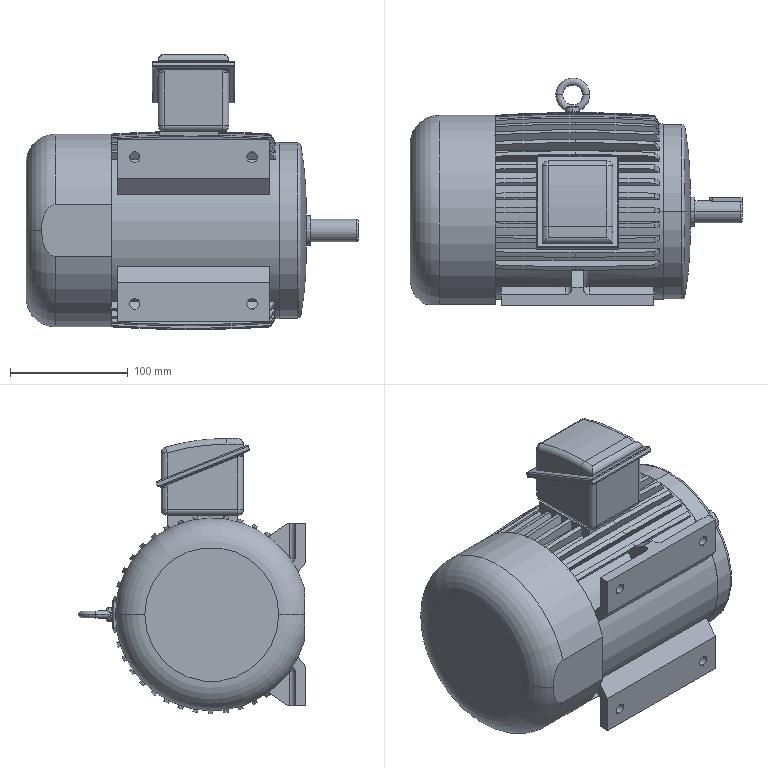Part | SolidWorks | features ICE 14, Fillet 10, CirPattern 2, Revolution 2, MirrorPattern 1, Shell 1, Sweep 1 | 5 solids | 377 faces | box 282.5 x 193.757 x 234.166 mm | volume 4079530 mm3 | plane 207 | cylinder 123 | torus 31 | spline 10 | sphere 6 | commonest cylinder face diameters 2000 x58 10 x20 2 x17 9 x8 149 x4 6 x2